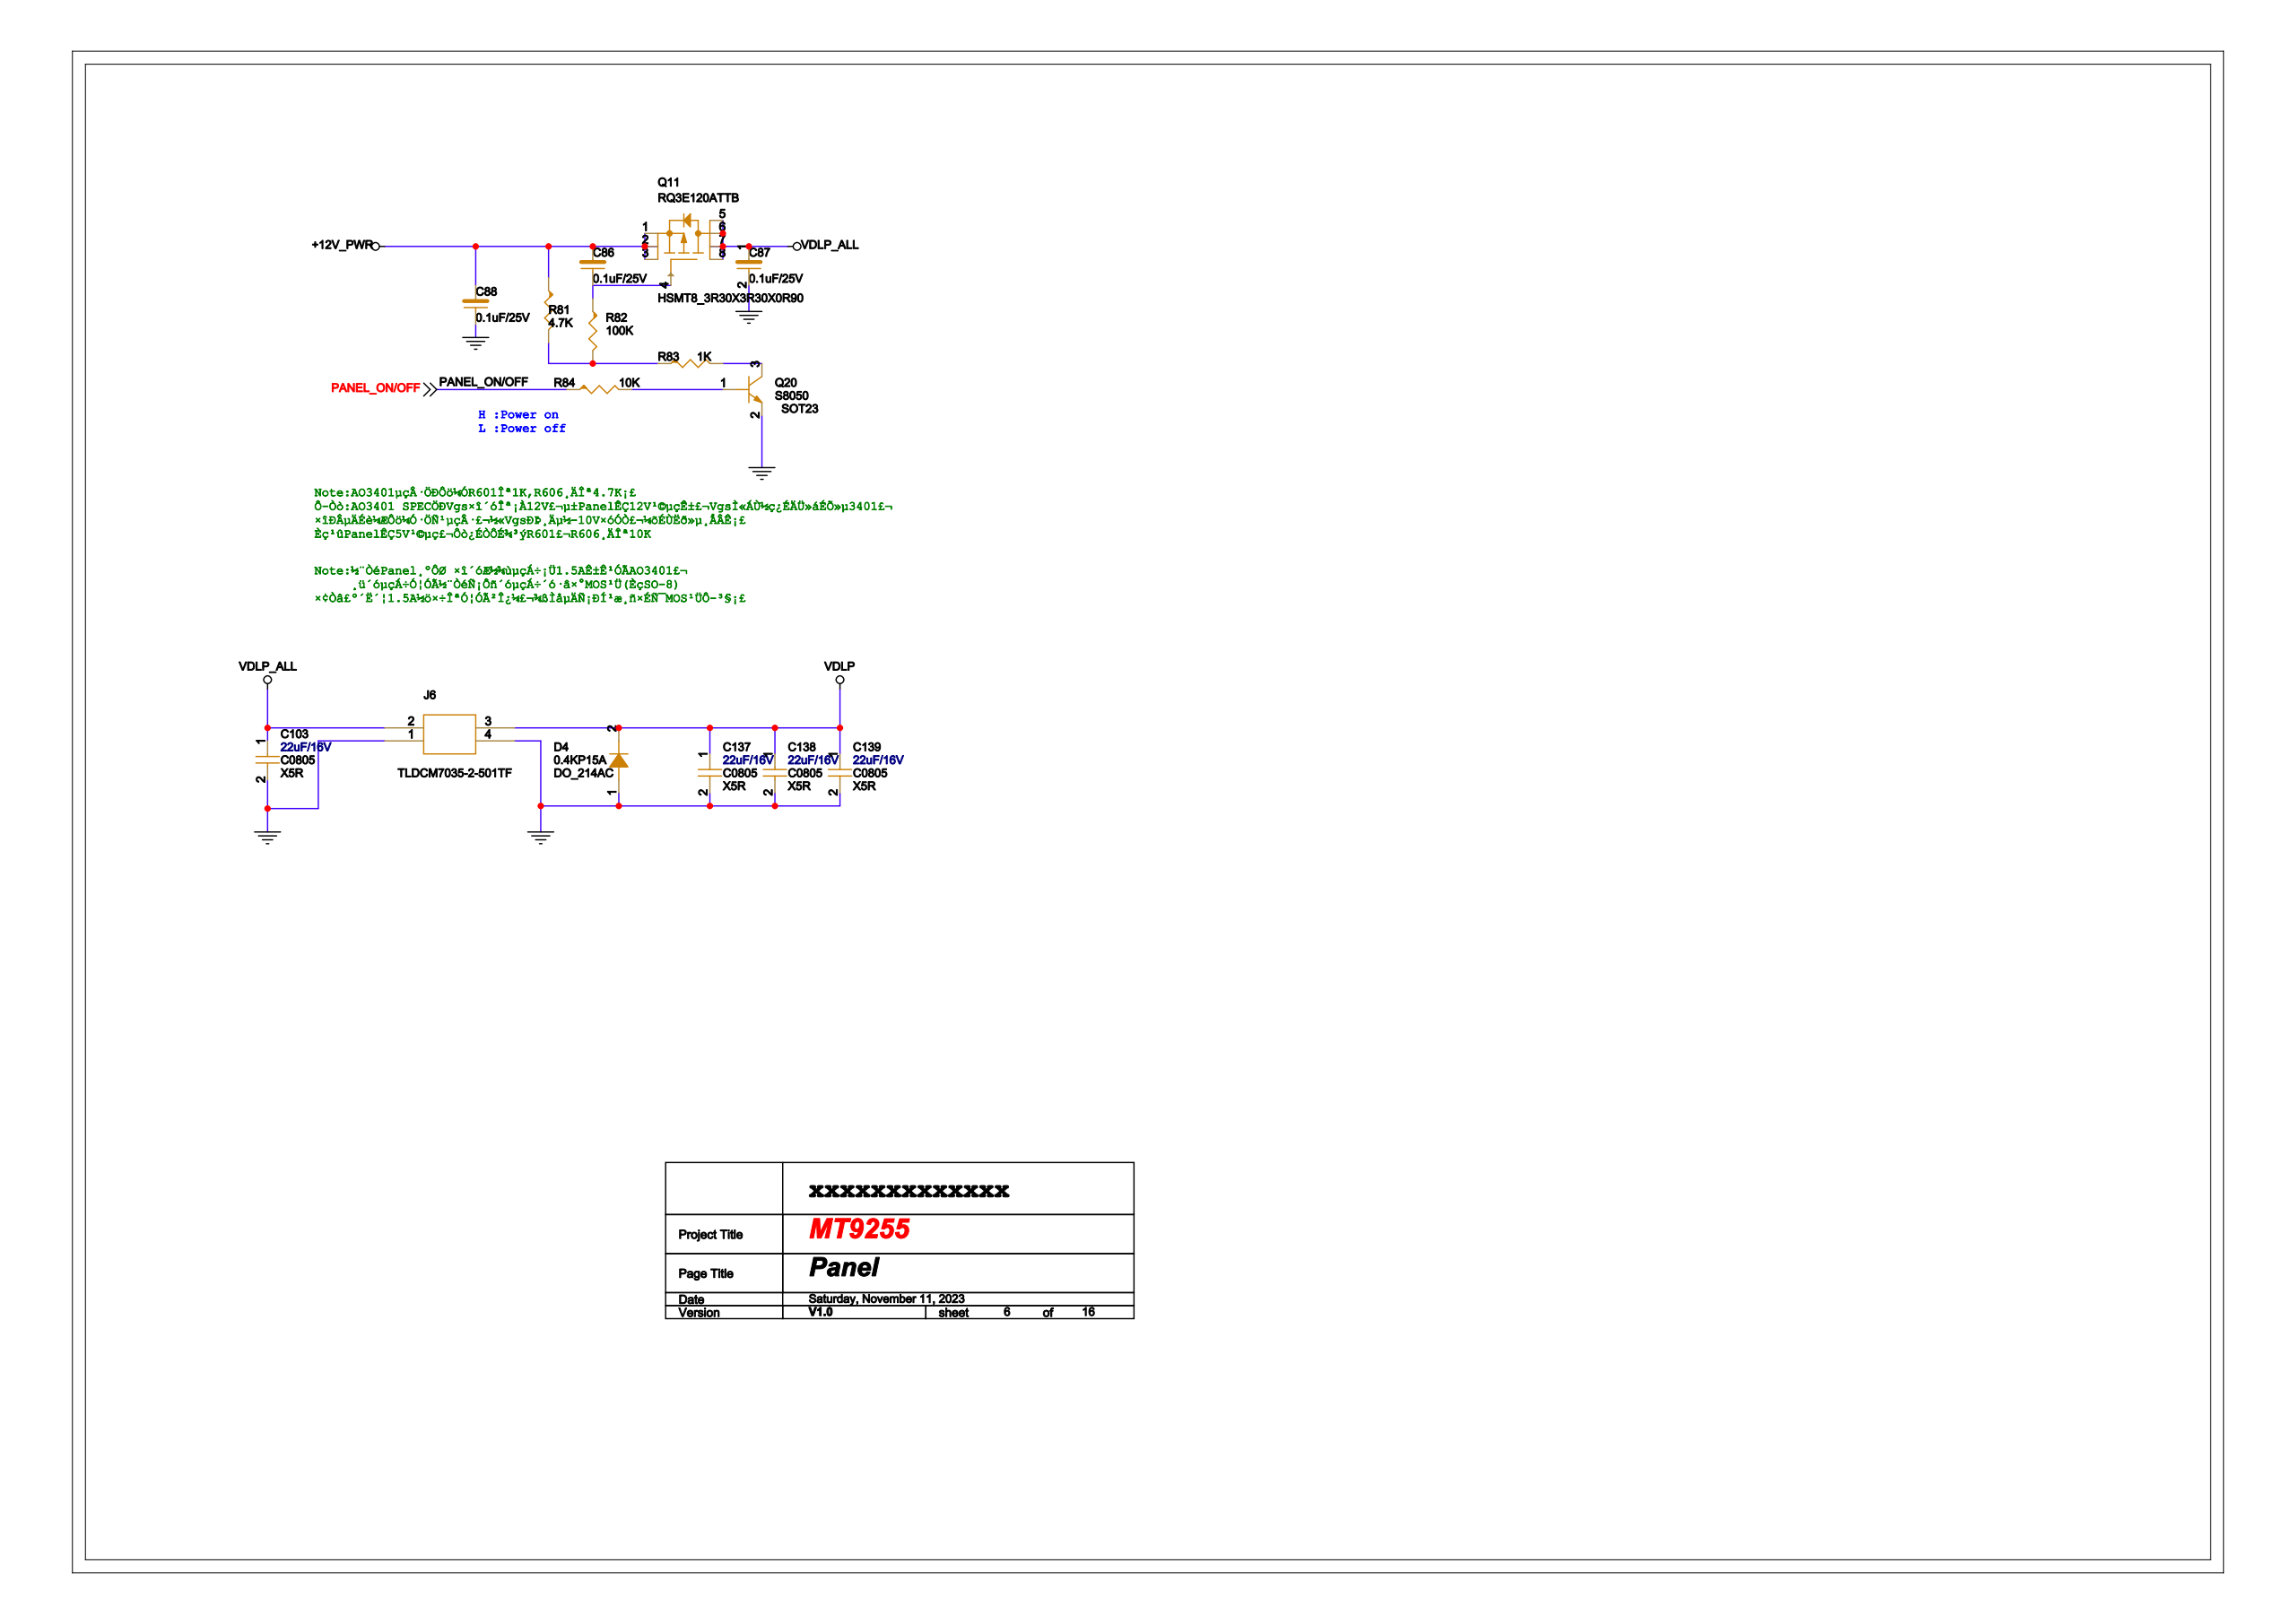Circuit board | Cadence Allegro | 1223 parts | 777 nets | one sheet of the schematic
Parts on this sheet (reference | value | footprint):
C86 | 0.1uF/25V | C0402
C87 | 0.1uF/25V | C0402
C88 | 0.1uF/25V | C0402
C103 | 22uF/16V | C0805
C137 | 22uF/16V | C0805
C138 | 22uF/16V | C0805
C139 | 22uF/16V | C0805
D4 | 0.4KP15A | DO_214AC
J6 | TLDCM7035-2-501TF | TLDCM7035
Q11 | RQ3E120ATTB | HSMT8_3R30X3R30X0R90
Q20 | S8050 | SOT23
R81 | 4.7K | R0402
R82 | 100K | R0402
R83 | 1K | R0402
R84 | 10K | R0402
Nets of these parts (net: part-pin ...):
GND: C87-2 C88-2 C103-2 C137-2 C138-2 C139-2 D4-1 J6-1 J6-4 Q20-2
+12V_PWR: C86-1 C88-1 Q11-1 Q11-2 Q11-3 R81-1
VDLP_ALL: C87-1 C103-1 J6-2 Q11-5 Q11-6 Q11-7 Q11-8
VDLP: C137-1 C138-1 C139-1 D4-2 J6-3
N21673863: C86-2 Q11-4 R82-1
N21675295: Q20-1 R84-2
N21675306: Q20-3 R83-2
PANEL_ON/OFF: R84-1
N21673735: R81-2 R82-2 R83-1